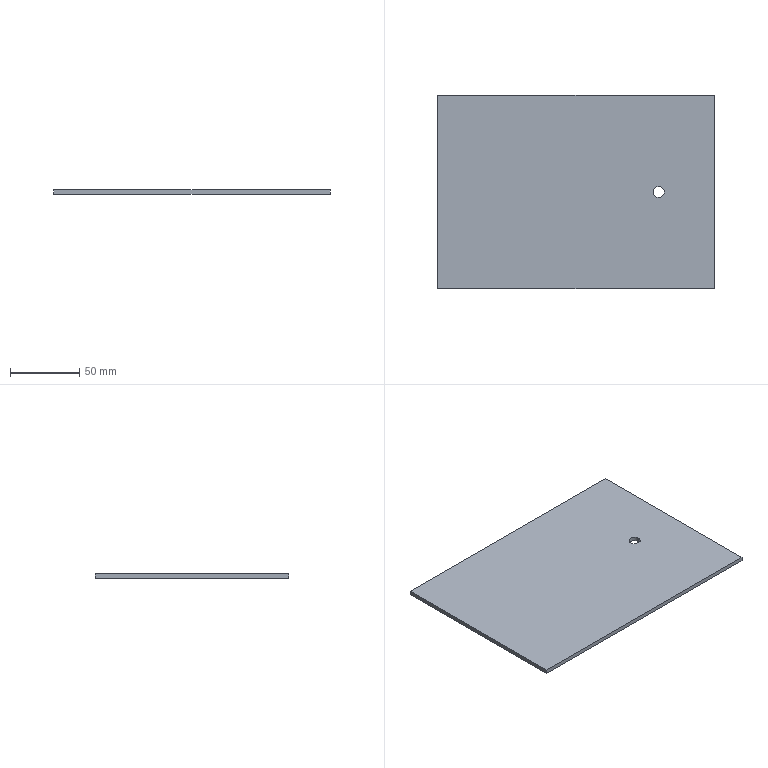Part | SolidWorks | features Extrusion 1, ICE 1 | 1 solid | 8 faces | box 200 x 140 x 3 mm | volume 83849 mm3 | plane 6 | cylinder 2 | commonest cylinder face diameters 8 x2
STEP:
#1=CARTESIAN_POINT('',(56.,0.,-1.5));
#2=VERTEX_POINT('',#1);
#3=CARTESIAN_POINT('',(64.,0.,-1.5));
#4=VERTEX_POINT('',#3);
#5=CARTESIAN_POINT('',(60.,0.,-1.5));
#6=DIRECTION('',(0.,0.,1.));
#7=DIRECTION('',(1.,0.,0.));
#8=AXIS2_PLACEMENT_3D('',#5,#6,#7);
#9=CIRCLE('',#8,4.);
#10=EDGE_CURVE('',#2,#4,#9,.T.);
#11=ORIENTED_EDGE('',*,*,#10,.F.);
#12=CARTESIAN_POINT('',(56.,0.,1.5));
#13=VERTEX_POINT('',#12);
#14=CARTESIAN_POINT('',(56.,0.,-11.5));
#15=DIRECTION('',(0.,0.,1.));
#16=VECTOR('',#15,1000.);
#17=LINE('',#14,#16);
#18=EDGE_CURVE('',#2,#13,#17,.T.);
#19=ORIENTED_EDGE('',*,*,#18,.T.);
#20=CARTESIAN_POINT('',(64.,0.,1.5));
#21=VERTEX_POINT('',#20);
#22=CARTESIAN_POINT('',(60.,0.,1.5));
#23=DIRECTION('',(0.,0.,1.));
#24=DIRECTION('',(1.,0.,0.));
#25=AXIS2_PLACEMENT_3D('',#22,#23,#24);
#26=CIRCLE('',#25,4.);
#27=EDGE_CURVE('',#13,#21,#26,.T.);
#28=ORIENTED_EDGE('',*,*,#27,.T.);
#29=CARTESIAN_POINT('',(64.,0.,-11.5));
#30=DIRECTION('',(0.,0.,1.));
#31=VECTOR('',#30,1000.);
#32=LINE('',#29,#31);
#33=EDGE_CURVE('',#4,#21,#32,.T.);
#34=ORIENTED_EDGE('',*,*,#33,.F.);
#35=EDGE_LOOP('',(#11,#19,#28,#34));
#36=FACE_OUTER_BOUND('',#35,.T.);
#37=CARTESIAN_POINT('',(60.,0.,-11.5));
#38=DIRECTION('',(0.,0.,1.));
#39=DIRECTION('',(1.,0.,0.));
#40=AXIS2_PLACEMENT_3D('',#37,#38,#39);
#41=CYLINDRICAL_SURFACE('',#40,4.);
#42=ADVANCED_FACE('',(#36),#41,.F.);
#43=CARTESIAN_POINT('',(-100.,70.,1.5));
#44=VERTEX_POINT('',#43);
#45=CARTESIAN_POINT('',(-100.,-70.,1.5));
#46=VERTEX_POINT('',#45);
#47=CARTESIAN_POINT('',(-100.,70.,1.5));
#48=DIRECTION('',(0.,-1.,0.));
#49=VECTOR('',#48,1000.);
#50=LINE('',#47,#49);
#51=EDGE_CURVE('',#44,#46,#50,.T.);
#52=ORIENTED_EDGE('',*,*,#51,.F.);
#53=CARTESIAN_POINT('',(-100.,70.,-1.5));
#54=VERTEX_POINT('',#53);
#55=CARTESIAN_POINT('',(-100.,70.,-1.5));
#56=DIRECTION('',(0.,0.,1.));
#57=VECTOR('',#56,1000.);
#58=LINE('',#55,#57);
#59=EDGE_CURVE('',#54,#44,#58,.T.);
#60=ORIENTED_EDGE('',*,*,#59,.F.);
#61=CARTESIAN_POINT('',(-100.,-70.,-1.5));
#62=VERTEX_POINT('',#61);
#63=CARTESIAN_POINT('',(-100.,70.,-1.5));
#64=DIRECTION('',(0.,-1.,0.));
#65=VECTOR('',#64,1000.);
#66=LINE('',#63,#65);
#67=EDGE_CURVE('',#54,#62,#66,.T.);
#68=ORIENTED_EDGE('',*,*,#67,.T.);
#69=CARTESIAN_POINT('',(-100.,-70.,-1.5));
#70=DIRECTION('',(0.,0.,1.));
#71=VECTOR('',#70,1000.);
#72=LINE('',#69,#71);
#73=EDGE_CURVE('',#62,#46,#72,.T.);
#74=ORIENTED_EDGE('',*,*,#73,.T.);
#75=EDGE_LOOP('',(#52,#60,#68,#74));
#76=FACE_OUTER_BOUND('',#75,.T.);
#77=CARTESIAN_POINT('',(-100.,70.,-1.5));
#78=DIRECTION('',(-1.,0.,0.));
#79=DIRECTION('',(0.,0.,1.));
#80=AXIS2_PLACEMENT_3D('',#77,#78,#79);
#81=PLANE('',#80);
#82=ADVANCED_FACE('',(#76),#81,.T.);
#83=CARTESIAN_POINT('',(100.,70.,1.5));
#84=VERTEX_POINT('',#83);
#85=CARTESIAN_POINT('',(100.,70.,1.5));
#86=DIRECTION('',(-1.,0.,0.));
#87=VECTOR('',#86,1000.);
#88=LINE('',#85,#87);
#89=EDGE_CURVE('',#84,#44,#88,.T.);
#90=ORIENTED_EDGE('',*,*,#89,.F.);
#91=CARTESIAN_POINT('',(100.,70.,-1.5));
#92=VERTEX_POINT('',#91);
#93=CARTESIAN_POINT('',(100.,70.,-1.5));
#94=DIRECTION('',(0.,0.,1.));
#95=VECTOR('',#94,1000.);
#96=LINE('',#93,#95);
#97=EDGE_CURVE('',#92,#84,#96,.T.);
#98=ORIENTED_EDGE('',*,*,#97,.F.);
#99=CARTESIAN_POINT('',(100.,70.,-1.5));
#100=DIRECTION('',(-1.,0.,0.));
#101=VECTOR('',#100,1000.);
#102=LINE('',#99,#101);
#103=EDGE_CURVE('',#92,#54,#102,.T.);
#104=ORIENTED_EDGE('',*,*,#103,.T.);
#105=ORIENTED_EDGE('',*,*,#59,.T.);
#106=EDGE_LOOP('',(#90,#98,#104,#105));
#107=FACE_OUTER_BOUND('',#106,.T.);
#108=CARTESIAN_POINT('',(100.,70.,-1.5));
#109=DIRECTION('',(0.,1.,0.));
#110=DIRECTION('',(0.,0.,1.));
#111=AXIS2_PLACEMENT_3D('',#108,#109,#110);
#112=PLANE('',#111);
#113=ADVANCED_FACE('',(#107),#112,.T.);
#114=CARTESIAN_POINT('',(100.,-70.,1.5));
#115=VERTEX_POINT('',#114);
#116=CARTESIAN_POINT('',(100.,-70.,1.5));
#117=DIRECTION('',(0.,1.,0.));
#118=VECTOR('',#117,1000.);
#119=LINE('',#116,#118);
#120=EDGE_CURVE('',#115,#84,#119,.T.);
#121=ORIENTED_EDGE('',*,*,#120,.F.);
#122=CARTESIAN_POINT('',(100.,-70.,-1.5));
#123=VERTEX_POINT('',#122);
#124=CARTESIAN_POINT('',(100.,-70.,-1.5));
#125=DIRECTION('',(0.,0.,1.));
#126=VECTOR('',#125,1000.);
#127=LINE('',#124,#126);
#128=EDGE_CURVE('',#123,#115,#127,.T.);
#129=ORIENTED_EDGE('',*,*,#128,.F.);
#130=CARTESIAN_POINT('',(100.,-70.,-1.5));
#131=DIRECTION('',(0.,1.,0.));
#132=VECTOR('',#131,1000.);
#133=LINE('',#130,#132);
#134=EDGE_CURVE('',#123,#92,#133,.T.);
#135=ORIENTED_EDGE('',*,*,#134,.T.);
#136=ORIENTED_EDGE('',*,*,#97,.T.);
#137=EDGE_LOOP('',(#121,#129,#135,#136));
#138=FACE_OUTER_BOUND('',#137,.T.);
#139=CARTESIAN_POINT('',(100.,-70.,-1.5));
#140=DIRECTION('',(1.,0.,0.));
#141=DIRECTION('',(0.,0.,-1.));
#142=AXIS2_PLACEMENT_3D('',#139,#140,#141);
#143=PLANE('',#142);
#144=ADVANCED_FACE('',(#138),#143,.T.);
#145=CARTESIAN_POINT('',(-100.,-70.,1.5));
#146=DIRECTION('',(1.,0.,0.));
#147=VECTOR('',#146,1000.);
#148=LINE('',#145,#147);
#149=EDGE_CURVE('',#46,#115,#148,.T.);
#150=ORIENTED_EDGE('',*,*,#149,.F.);
#151=ORIENTED_EDGE('',*,*,#73,.F.);
#152=CARTESIAN_POINT('',(-100.,-70.,-1.5));
#153=DIRECTION('',(1.,0.,0.));
#154=VECTOR('',#153,1000.);
#155=LINE('',#152,#154);
#156=EDGE_CURVE('',#62,#123,#155,.T.);
#157=ORIENTED_EDGE('',*,*,#156,.T.);
#158=ORIENTED_EDGE('',*,*,#128,.T.);
#159=EDGE_LOOP('',(#150,#151,#157,#158));
#160=FACE_OUTER_BOUND('',#159,.T.);
#161=CARTESIAN_POINT('',(-100.,-70.,-1.5));
#162=DIRECTION('',(0.,-1.,0.));
#163=DIRECTION('',(0.,0.,-1.));
#164=AXIS2_PLACEMENT_3D('',#161,#162,#163);
#165=PLANE('',#164);
#166=ADVANCED_FACE('',(#160),#165,.T.);
#167=CARTESIAN_POINT('',(60.,0.,-1.5));
#168=DIRECTION('',(0.,0.,1.));
#169=DIRECTION('',(1.,0.,0.));
#170=AXIS2_PLACEMENT_3D('',#167,#168,#169);
#171=CIRCLE('',#170,4.);
#172=EDGE_CURVE('',#4,#2,#171,.T.);
#173=ORIENTED_EDGE('',*,*,#172,.T.);
#174=ORIENTED_EDGE('',*,*,#10,.T.);
#175=EDGE_LOOP('',(#173,#174));
#176=FACE_BOUND('',#175,.T.);
#177=ORIENTED_EDGE('',*,*,#67,.F.);
#178=ORIENTED_EDGE('',*,*,#103,.F.);
#179=ORIENTED_EDGE('',*,*,#134,.F.);
#180=ORIENTED_EDGE('',*,*,#156,.F.);
#181=EDGE_LOOP('',(#177,#178,#179,#180));
#182=FACE_OUTER_BOUND('',#181,.T.);
#183=CARTESIAN_POINT('',(0.,0.,-1.5));
#184=DIRECTION('',(0.,0.,1.));
#185=DIRECTION('',(1.,0.,0.));
#186=AXIS2_PLACEMENT_3D('',#183,#184,#185);
#187=PLANE('',#186);
#188=ADVANCED_FACE('',(#176,#182),#187,.F.);
#189=CARTESIAN_POINT('',(60.,0.,1.5));
#190=DIRECTION('',(0.,0.,1.));
#191=DIRECTION('',(1.,0.,0.));
#192=AXIS2_PLACEMENT_3D('',#189,#190,#191);
#193=CIRCLE('',#192,4.);
#194=EDGE_CURVE('',#21,#13,#193,.T.);
#195=ORIENTED_EDGE('',*,*,#194,.F.);
#196=ORIENTED_EDGE('',*,*,#27,.F.);
#197=EDGE_LOOP('',(#195,#196));
#198=FACE_BOUND('',#197,.T.);
#199=ORIENTED_EDGE('',*,*,#51,.T.);
#200=ORIENTED_EDGE('',*,*,#149,.T.);
#201=ORIENTED_EDGE('',*,*,#120,.T.);
#202=ORIENTED_EDGE('',*,*,#89,.T.);
#203=EDGE_LOOP('',(#199,#200,#201,#202));
#204=FACE_OUTER_BOUND('',#203,.T.);
#205=CARTESIAN_POINT('',(0.,0.,1.5));
#206=DIRECTION('',(0.,0.,1.));
#207=DIRECTION('',(1.,0.,0.));
#208=AXIS2_PLACEMENT_3D('',#205,#206,#207);
#209=PLANE('',#208);
#210=ADVANCED_FACE('',(#198,#204),#209,.T.);
#211=ORIENTED_EDGE('',*,*,#18,.F.);
#212=ORIENTED_EDGE('',*,*,#172,.F.);
#213=ORIENTED_EDGE('',*,*,#33,.T.);
#214=ORIENTED_EDGE('',*,*,#194,.T.);
#215=EDGE_LOOP('',(#211,#212,#213,#214));
#216=FACE_OUTER_BOUND('',#215,.T.);
#217=CARTESIAN_POINT('',(60.,0.,-11.5));
#218=DIRECTION('',(0.,0.,1.));
#219=DIRECTION('',(1.,0.,0.));
#220=AXIS2_PLACEMENT_3D('',#217,#218,#219);
#221=CYLINDRICAL_SURFACE('',#220,4.);
#222=ADVANCED_FACE('',(#216),#221,.F.);
#223=CLOSED_SHELL('',(#42,#82,#113,#144,#166,#188,#210,#222));
#224=MANIFOLD_SOLID_BREP('',#223);
#225=CARTESIAN_POINT('',(0.,0.,0.));
#226=DIRECTION('',(0.,0.,1.));
#227=DIRECTION('',(1.,0.,0.));
#228=AXIS2_PLACEMENT_3D('',#225,#226,#227);
#229=(LENGTH_UNIT()NAMED_UNIT(*)SI_UNIT(.MILLI.,.METRE.));
#230=UNCERTAINTY_MEASURE_WITH_UNIT(LENGTH_MEASURE(0.00001),#229,'','');
#231=(NAMED_UNIT(*)PLANE_ANGLE_UNIT()SI_UNIT($,.RADIAN.));
#232=(NAMED_UNIT(*)SI_UNIT($,.STERADIAN.)SOLID_ANGLE_UNIT());
#233=(GEOMETRIC_REPRESENTATION_CONTEXT(3)GLOBAL_UNCERTAINTY_ASSIGNED_CONTEXT((#230))GLOBAL_UNIT_ASSIGNED_CONTEXT((#229,#231,#232))REPRESENTATION_CONTEXT('',''));
#234=ADVANCED_BREP_SHAPE_REPRESENTATION('',(#224,#228),#233);